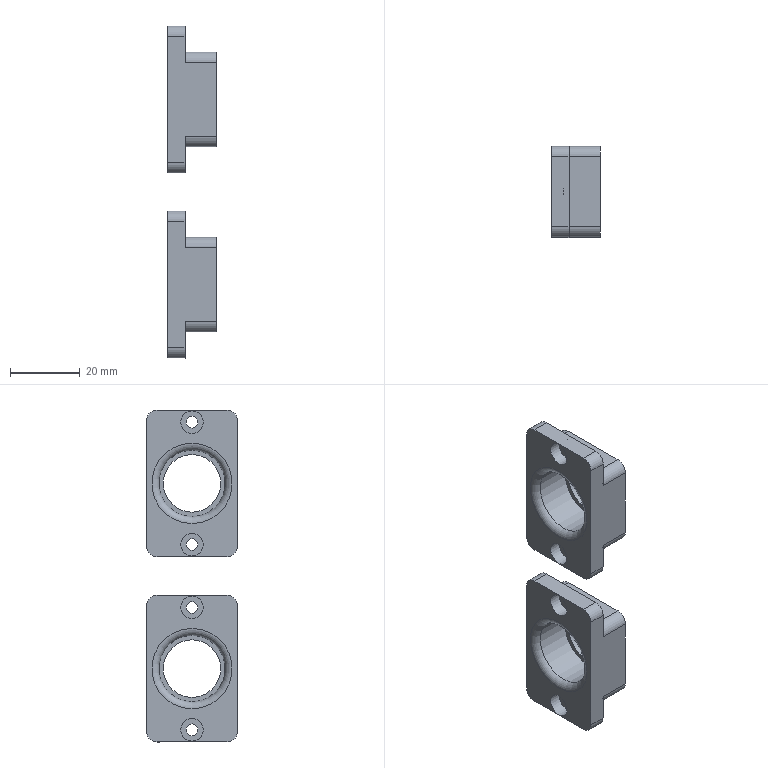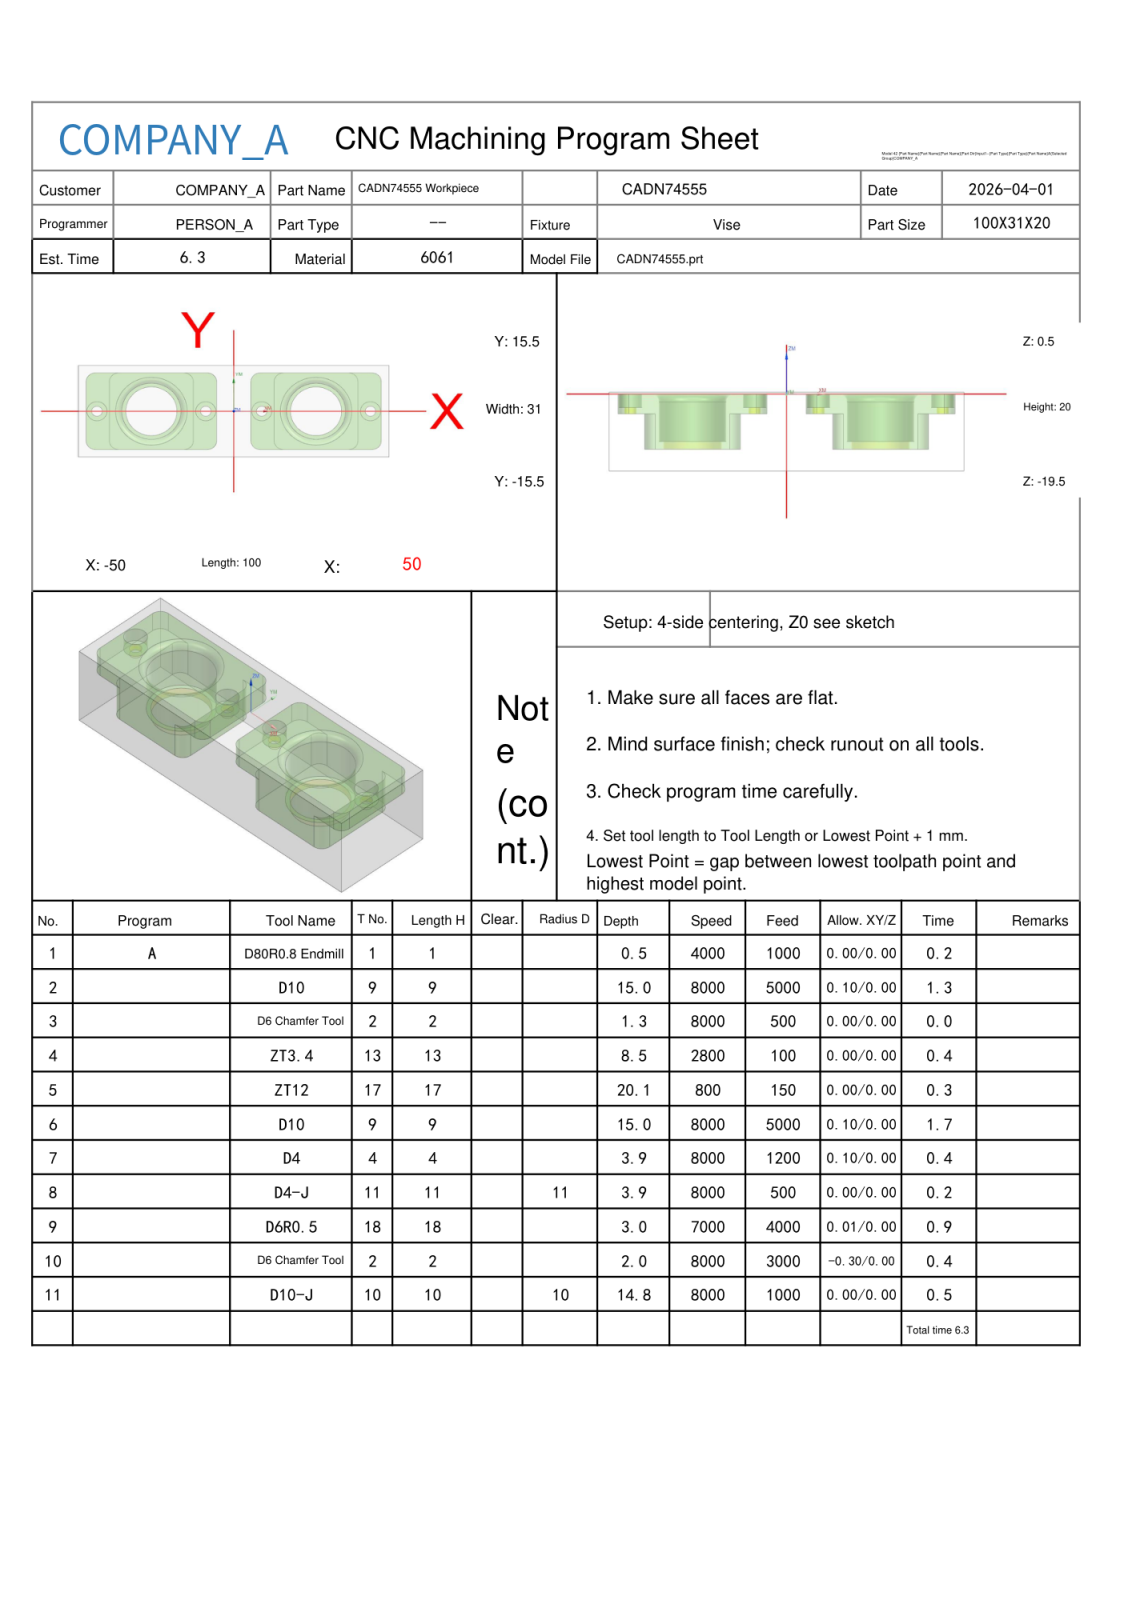NC program | NX | posted by the shop | part box 14 x 26 x 95 mm
Lines 5365 to 5542 of 19918:
N7 T04 M06
(D4  D=4. R=0. H=04 ce=0.10 di=0.00)
G00 G90 G54 X-9. Y0.0 M03 S8000
G43 H04 Z20.
M08
Z.5
G03 X-9.575 Y-.575 I0.0 J-.575 F1200.
X-9. Y-1.15 I.575 J0.0
X-9. Y-1.15 Z.2 I0.0 J1.15
X-9. Y-1.15 Z-.1 I0.0 J1.15
X-9. Y-1.15 Z-.4 I0.0 J1.15
X-9. Y-1.15 Z-.7 I0.0 J1.15
X-9. Y-1.15 Z-1. I0.0 J1.15
X-9. Y-1.15 Z-1.3 I0.0 J1.15
X-9. Y-1.15 Z-1.6 I0.0 J1.15
X-9. Y-1.15 Z-1.9 I0.0 J1.15
X-9. Y-1.15 Z-2.2 I0.0 J1.15
X-9. Y-1.15 Z-2.5 I0.0 J1.15
X-9. Y-1.15 Z-2.8 I0.0 J1.15
X-9. Y-1.15 Z-3.1 I0.0 J1.15
X-9. Y-1.15 Z-3.4 I0.0 J1.15
X-7.85 Y0.0 I0.0 J1.15
X-9. Y1.15 I-1.15 J0.0
X-10.15 Y0.0 I0.0 J-1.15
X-9. Y-1.15 I1.15 J0.0
X-8.425 Y-.575 I0.0 J.575
X-9. Y0.0 I-.575 J0.0
G00 Z20.
X-44.
Z.5
G03 X-44.575 Y-.575 I0.0 J-.575
X-44. Y-1.15 I.575 J0.0
X-44. Y-1.15 Z.2 I0.0 J1.15
X-44. Y-1.15 Z-.1 I0.0 J1.15
X-44. Y-1.15 Z-.4 I0.0 J1.15
X-44. Y-1.15 Z-.7 I0.0 J1.15
X-44. Y-1.15 Z-1. I0.0 J1.15
X-44. Y-1.15 Z-1.3 I0.0 J1.15
X-44. Y-1.15 Z-1.6 I0.0 J1.15
X-44. Y-1.15 Z-1.9 I0.0 J1.15
X-44. Y-1.15 Z-2.2 I0.0 J1.15
X-44. Y-1.15 Z-2.5 I0.0 J1.15
X-44. Y-1.15 Z-2.8 I0.0 J1.15
X-44. Y-1.15 Z-3.1 I0.0 J1.15
X-44. Y-1.15 Z-3.4 I0.0 J1.15
X-42.85 Y0.0 I0.0 J1.15
X-44. Y1.15 I-1.15 J0.0
X-45.15 Y0.0 I0.0 J-1.15
X-44. Y-1.15 I1.15 J0.0
X-43.425 Y-.575 I0.0 J.575
X-44. Y0.0 I-.575 J0.0
G00 Z20.
X9.
Z.5
G03 X8.425 Y-.575 I0.0 J-.575
X9. Y-1.15 I.575 J0.0
X9. Y-1.15 Z.2 I0.0 J1.15
X9. Y-1.15 Z-.1 I0.0 J1.15
X9. Y-1.15 Z-.4 I0.0 J1.15
X9. Y-1.15 Z-.7 I0.0 J1.15
X9. Y-1.15 Z-1. I0.0 J1.15
X9. Y-1.15 Z-1.3 I0.0 J1.15
X9. Y-1.15 Z-1.6 I0.0 J1.15
X9. Y-1.15 Z-1.9 I0.0 J1.15
X9. Y-1.15 Z-2.2 I0.0 J1.15
X9. Y-1.15 Z-2.5 I0.0 J1.15
X9. Y-1.15 Z-2.8 I0.0 J1.15
X9. Y-1.15 Z-3.1 I0.0 J1.15
X9. Y-1.15 Z-3.4 I0.0 J1.15
X10.15 Y0.0 I0.0 J1.15
X9. Y1.15 I-1.15 J0.0
X7.85 Y0.0 I0.0 J-1.15
X9. Y-1.15 I1.15 J0.0
X9.575 Y-.575 I0.0 J.575
X9. Y0.0 I-.575 J0.0
G00 Z20.
X44.
Z.5
G03 X43.425 Y-.575 I0.0 J-.575
X44. Y-1.15 I.575 J0.0
X44. Y-1.15 Z.2 I0.0 J1.15
X44. Y-1.15 Z-.1 I0.0 J1.15
X44. Y-1.15 Z-.4 I0.0 J1.15
X44. Y-1.15 Z-.7 I0.0 J1.15
X44. Y-1.15 Z-1. I0.0 J1.15
X44. Y-1.15 Z-1.3 I0.0 J1.15
X44. Y-1.15 Z-1.6 I0.0 J1.15
X44. Y-1.15 Z-1.9 I0.0 J1.15
X44. Y-1.15 Z-2.2 I0.0 J1.15
X44. Y-1.15 Z-2.5 I0.0 J1.15
X44. Y-1.15 Z-2.8 I0.0 J1.15
X44. Y-1.15 Z-3.1 I0.0 J1.15
X44. Y-1.15 Z-3.4 I0.0 J1.15
X45.15 Y0.0 I0.0 J1.15
X44. Y1.15 I-1.15 J0.0
X42.85 Y0.0 I0.0 J-1.15
X44. Y-1.15 I1.15 J0.0
X44.575 Y-.575 I0.0 J.575
X44. Y0.0 I-.575 J0.0
G00 Z20.
G91 G28 Z0.0
M05
M09
G91 G28 Z0.0
M01
N8 T11 M06
(D4-J  D=4. R=0. H=11 ce=0.00 di=0.00)
G00 G90 G54 X-9. Y0.0 M03 S8000
G43 H11 Z20.
M08
Z.5
G41 D11
G01 X-9.19 Y-.062 F500.
G03 X-9.609 Y-.641 I.19 J-.579
X-9. Y-1.25 I.609 J0.0
X-10.228 Y-.234 Z-3.4 I0.0 J1.25
X-9. Y-1.25 I1.228 J.234
X-7.75 Y0.0 I0.0 J1.25
X-9. Y1.25 I-1.25 J0.0
X-10.25 Y0.0 I0.0 J-1.25
X-10.228 Y-.234 I1.25 J0.0
X-9.63 Y-.729 I.598 J.114
X-9.026 Y-.198 I0.0 J.609
G01 G40 X-9. Y0.0
G00 Z20.
X-44.
Z.5
G41 D11
G01 X-44.19 Y-.062
G03 X-44.609 Y-.641 I.19 J-.579
X-44. Y-1.25 I.609 J0.0
X-45.228 Y-.234 Z-3.4 I0.0 J1.25
X-44. Y-1.25 I1.228 J.234
X-42.75 Y0.0 I0.0 J1.25
X-44. Y1.25 I-1.25 J0.0
X-45.25 Y0.0 I0.0 J-1.25
X-45.228 Y-.234 I1.25 J0.0
X-44.63 Y-.729 I.598 J.114
X-44.026 Y-.198 I0.0 J.609
G01 G40 X-44. Y0.0
G00 Z20.
X9.
Z.5
G41 D11
G01 X8.81 Y-.062
G03 X8.391 Y-.641 I.19 J-.579
X9. Y-1.25 I.609 J0.0
X7.772 Y-.234 Z-3.4 I0.0 J1.25
X9. Y-1.25 I1.228 J.234
X10.25 Y0.0 I0.0 J1.25
X9. Y1.25 I-1.25 J0.0
X7.75 Y0.0 I0.0 J-1.25
X7.772 Y-.234 I1.25 J0.0
X8.37 Y-.729 I.598 J.114
X8.974 Y-.198 I0.0 J.609
G01 G40 X9. Y0.0
G00 Z20.
X44.
Z.5
G41 D11
G01 X43.81 Y-.062
G03 X43.391 Y-.641 I.19 J-.579
X44. Y-1.25 I.609 J0.0
X42.772 Y-.234 Z-3.4 I0.0 J1.25
X44. Y-1.25 I1.228 J.234
X45.25 Y0.0 I0.0 J1.25
X44. Y1.25 I-1.25 J0.0
X42.75 Y0.0 I0.0 J-1.25
X42.772 Y-.234 I1.25 J0.0
X43.37 Y-.729 I.598 J.114
X43.974 Y-.198 I0.0 J.609
G01 G40 X44. Y0.0
G00 Z20.
G91 G28 Z0.0
M05
M09
G91 G28 Z0.0
M01